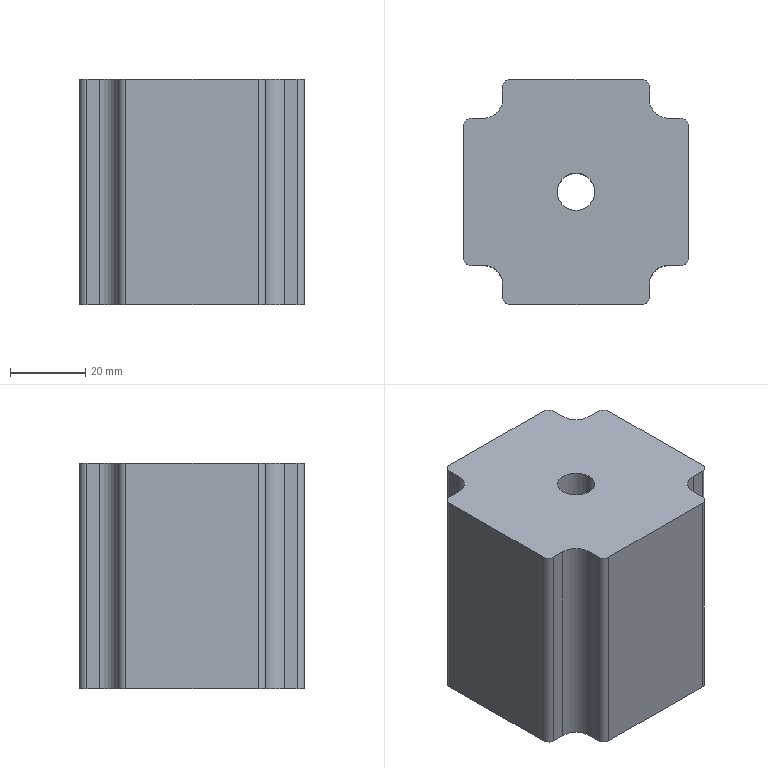Part | STEP file | 31090521--MS1H1-400001_1_1_1 | 1 solid | 34 faces | box 60 x 60 x 60 mm | volume 186186 mm3 | cylinder 18 | plane 16 | commonest cylinder face diameters 4 x8 10 x6 2 x4